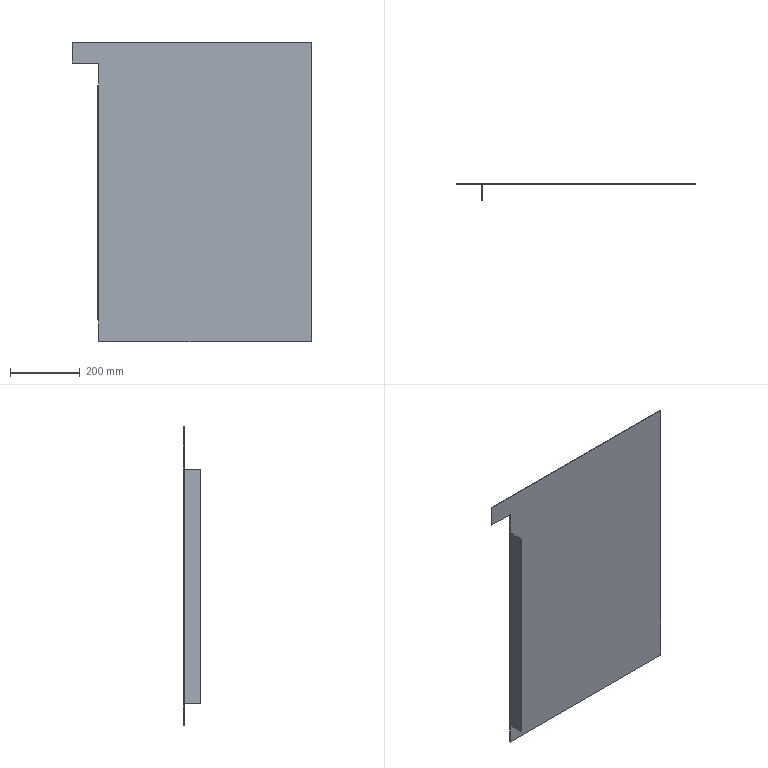Part | STEP file | 楼梯踏Plate 3 | 1 solid | 16 faces | box 686 x 50 x 860 mm | volume 1690832 mm3 | plane 14 | cylinder 2 | commonest cylinder face diameters 2 x1 8 x1
STEP:
#1=CARTESIAN_POINT('',(0.,0.,0.));
#2=DIRECTION('',(0.,0.,1.));
#3=DIRECTION('',(1.,0.,0.));
#4=AXIS2_PLACEMENT_3D('',#1,#2,#3);
#5=CARTESIAN_POINT('',(-611.,-3.,337.));
#6=VERTEX_POINT('',#5);
#7=CARTESIAN_POINT('',(-611.,-3.,-337.));
#8=VERTEX_POINT('',#7);
#9=CARTESIAN_POINT('',(-611.,-3.,337.));
#10=DIRECTION('',(0.,0.,-1.));
#11=VECTOR('',#10,1.);
#12=LINE('',#9,#11);
#13=CARTESIAN_POINT('',(-611.,-3.,337.));
#14=DIRECTION('',(0.,1.,0.));
#15=DIRECTION('',(0.,0.,1.));
#16=AXIS2_PLACEMENT_3D('',#13,#14,#15);
#17=PLANE('',#16);
#18=CARTESIAN_POINT('',(0.,0.));
#19=DIRECTION('',(-1.,0.));
#20=VECTOR('',#19,1.);
#21=LINE('',#18,#20);
#22=(GEOMETRIC_REPRESENTATION_CONTEXT(2)PARAMETRIC_REPRESENTATION_CONTEXT()REPRESENTATION_CONTEXT('',''));
#23=DEFINITIONAL_REPRESENTATION('',(#21),#22);
#24=PCURVE('',#17,#23);
#25=CARTESIAN_POINT('',(-611.,-4.,337.));
#26=DIRECTION('',(0.,0.,-1.));
#27=DIRECTION('',(-1.,0.,0.));
#28=AXIS2_PLACEMENT_3D('',#25,#26,#27);
#29=CYLINDRICAL_SURFACE('',#28,1.);
#30=CARTESIAN_POINT('',(1.571,0.));
#31=DIRECTION('',(0.,1.));
#32=VECTOR('',#31,1.);
#33=LINE('',#30,#32);
#34=(GEOMETRIC_REPRESENTATION_CONTEXT(2)PARAMETRIC_REPRESENTATION_CONTEXT()REPRESENTATION_CONTEXT('',''));
#35=DEFINITIONAL_REPRESENTATION('',(#33),#34);
#36=PCURVE('',#29,#35);
#37=SURFACE_CURVE('',#12,(#24,#36),.PCURVE_S1.);
#38=EDGE_CURVE('',#6,#8,#37,.T.);
#39=ORIENTED_EDGE('',*,*,#38,.T.);
#40=CARTESIAN_POINT('',(-611.,-3.,-400.));
#41=VERTEX_POINT('',#40);
#42=CARTESIAN_POINT('',(-611.,-3.,-337.));
#43=DIRECTION('',(0.,0.,1.));
#44=VECTOR('',#43,1.);
#45=LINE('',#42,#44);
#46=CARTESIAN_POINT('',(-674.,0.));
#47=DIRECTION('',(1.,0.));
#48=VECTOR('',#47,1.);
#49=LINE('',#46,#48);
#50=(GEOMETRIC_REPRESENTATION_CONTEXT(2)PARAMETRIC_REPRESENTATION_CONTEXT()REPRESENTATION_CONTEXT('',''));
#51=DEFINITIONAL_REPRESENTATION('',(#49),#50);
#52=PCURVE('',#17,#51);
#53=CARTESIAN_POINT('',(-611.,-3.,-337.));
#54=DIRECTION('',(-1.,0.,0.));
#55=DIRECTION('',(0.,0.,1.));
#56=AXIS2_PLACEMENT_3D('',#53,#54,#55);
#57=PLANE('',#56);
#58=CARTESIAN_POINT('',(0.,0.));
#59=DIRECTION('',(1.,0.));
#60=VECTOR('',#59,1.);
#61=LINE('',#58,#60);
#62=(GEOMETRIC_REPRESENTATION_CONTEXT(2)PARAMETRIC_REPRESENTATION_CONTEXT()REPRESENTATION_CONTEXT('',''));
#63=DEFINITIONAL_REPRESENTATION('',(#61),#62);
#64=PCURVE('',#57,#63);
#65=SURFACE_CURVE('',#45,(#52,#64),.PCURVE_S1.);
#66=EDGE_CURVE('',#41,#8,#65,.T.);
#67=ORIENTED_EDGE('',*,*,#66,.F.);
#68=CARTESIAN_POINT('',(0.,-3.,-400.));
#69=VERTEX_POINT('',#68);
#70=CARTESIAN_POINT('',(-611.,-3.,-400.));
#71=DIRECTION('',(-1.,0.,0.));
#72=VECTOR('',#71,1.);
#73=LINE('',#70,#72);
#74=CARTESIAN_POINT('',(-737.,0.));
#75=DIRECTION('',(0.,-1.));
#76=VECTOR('',#75,1.);
#77=LINE('',#74,#76);
#78=(GEOMETRIC_REPRESENTATION_CONTEXT(2)PARAMETRIC_REPRESENTATION_CONTEXT()REPRESENTATION_CONTEXT('',''));
#79=DEFINITIONAL_REPRESENTATION('',(#77),#78);
#80=PCURVE('',#17,#79);
#81=CARTESIAN_POINT('',(-611.,-3.,-400.));
#82=DIRECTION('',(0.,0.,-1.));
#83=DIRECTION('',(-1.,0.,0.));
#84=AXIS2_PLACEMENT_3D('',#81,#82,#83);
#85=PLANE('',#84);
#86=CARTESIAN_POINT('',(0.,0.));
#87=DIRECTION('',(1.,0.));
#88=VECTOR('',#87,1.);
#89=LINE('',#86,#88);
#90=(GEOMETRIC_REPRESENTATION_CONTEXT(2)PARAMETRIC_REPRESENTATION_CONTEXT()REPRESENTATION_CONTEXT('',''));
#91=DEFINITIONAL_REPRESENTATION('',(#89),#90);
#92=PCURVE('',#85,#91);
#93=SURFACE_CURVE('',#73,(#80,#92),.PCURVE_S1.);
#94=EDGE_CURVE('',#69,#41,#93,.T.);
#95=ORIENTED_EDGE('',*,*,#94,.F.);
#96=CARTESIAN_POINT('',(0.,-3.,460.));
#97=VERTEX_POINT('',#96);
#98=CARTESIAN_POINT('',(0.,-3.,337.));
#99=DIRECTION('',(0.,0.,-1.));
#100=VECTOR('',#99,1.);
#101=LINE('',#98,#100);
#102=CARTESIAN_POINT('',(0.,611.));
#103=DIRECTION('',(-1.,0.));
#104=VECTOR('',#103,1.);
#105=LINE('',#102,#104);
#106=(GEOMETRIC_REPRESENTATION_CONTEXT(2)PARAMETRIC_REPRESENTATION_CONTEXT()REPRESENTATION_CONTEXT('',''));
#107=DEFINITIONAL_REPRESENTATION('',(#105),#106);
#108=PCURVE('',#17,#107);
#109=CARTESIAN_POINT('',(0.,0.,337.));
#110=DIRECTION('',(1.,0.,0.));
#111=DIRECTION('',(0.,0.,-1.));
#112=AXIS2_PLACEMENT_3D('',#109,#110,#111);
#113=PLANE('',#112);
#114=CARTESIAN_POINT('',(0.,-3.));
#115=DIRECTION('',(1.,0.));
#116=VECTOR('',#115,1.);
#117=LINE('',#114,#116);
#118=(GEOMETRIC_REPRESENTATION_CONTEXT(2)PARAMETRIC_REPRESENTATION_CONTEXT()REPRESENTATION_CONTEXT('',''));
#119=DEFINITIONAL_REPRESENTATION('',(#117),#118);
#120=PCURVE('',#113,#119);
#121=SURFACE_CURVE('',#101,(#108,#120),.PCURVE_S1.);
#122=EDGE_CURVE('',#97,#69,#121,.T.);
#123=ORIENTED_EDGE('',*,*,#122,.F.);
#124=CARTESIAN_POINT('',(-686.,-3.,460.));
#125=VERTEX_POINT('',#124);
#126=CARTESIAN_POINT('',(-611.,-3.,460.));
#127=DIRECTION('',(1.,0.,0.));
#128=VECTOR('',#127,1.);
#129=LINE('',#126,#128);
#130=CARTESIAN_POINT('',(123.,0.));
#131=DIRECTION('',(0.,1.));
#132=VECTOR('',#131,1.);
#133=LINE('',#130,#132);
#134=(GEOMETRIC_REPRESENTATION_CONTEXT(2)PARAMETRIC_REPRESENTATION_CONTEXT()REPRESENTATION_CONTEXT('',''));
#135=DEFINITIONAL_REPRESENTATION('',(#133),#134);
#136=PCURVE('',#17,#135);
#137=CARTESIAN_POINT('',(-611.,-3.,460.));
#138=DIRECTION('',(0.,0.,1.));
#139=DIRECTION('',(1.,0.,0.));
#140=AXIS2_PLACEMENT_3D('',#137,#138,#139);
#141=PLANE('',#140);
#142=CARTESIAN_POINT('',(0.,0.));
#143=DIRECTION('',(1.,0.));
#144=VECTOR('',#143,1.);
#145=LINE('',#142,#144);
#146=(GEOMETRIC_REPRESENTATION_CONTEXT(2)PARAMETRIC_REPRESENTATION_CONTEXT()REPRESENTATION_CONTEXT('',''));
#147=DEFINITIONAL_REPRESENTATION('',(#145),#146);
#148=PCURVE('',#141,#147);
#149=SURFACE_CURVE('',#129,(#136,#148),.PCURVE_S1.);
#150=EDGE_CURVE('',#125,#97,#149,.T.);
#151=ORIENTED_EDGE('',*,*,#150,.F.);
#152=CARTESIAN_POINT('',(-686.,-3.,400.));
#153=VERTEX_POINT('',#152);
#154=CARTESIAN_POINT('',(-686.,-3.,460.));
#155=DIRECTION('',(0.,0.,1.));
#156=VECTOR('',#155,1.);
#157=LINE('',#154,#156);
#158=CARTESIAN_POINT('',(123.,-75.));
#159=DIRECTION('',(1.,0.));
#160=VECTOR('',#159,1.);
#161=LINE('',#158,#160);
#162=(GEOMETRIC_REPRESENTATION_CONTEXT(2)PARAMETRIC_REPRESENTATION_CONTEXT()REPRESENTATION_CONTEXT('',''));
#163=DEFINITIONAL_REPRESENTATION('',(#161),#162);
#164=PCURVE('',#17,#163);
#165=CARTESIAN_POINT('',(-686.,-3.,460.));
#166=DIRECTION('',(-1.,0.,0.));
#167=DIRECTION('',(0.,0.,1.));
#168=AXIS2_PLACEMENT_3D('',#165,#166,#167);
#169=PLANE('',#168);
#170=CARTESIAN_POINT('',(0.,0.));
#171=DIRECTION('',(1.,0.));
#172=VECTOR('',#171,1.);
#173=LINE('',#170,#172);
#174=(GEOMETRIC_REPRESENTATION_CONTEXT(2)PARAMETRIC_REPRESENTATION_CONTEXT()REPRESENTATION_CONTEXT('',''));
#175=DEFINITIONAL_REPRESENTATION('',(#173),#174);
#176=PCURVE('',#169,#175);
#177=SURFACE_CURVE('',#157,(#164,#176),.PCURVE_S1.);
#178=EDGE_CURVE('',#153,#125,#177,.T.);
#179=ORIENTED_EDGE('',*,*,#178,.F.);
#180=CARTESIAN_POINT('',(-611.,-3.,400.));
#181=VERTEX_POINT('',#180);
#182=CARTESIAN_POINT('',(-611.,-3.,400.));
#183=DIRECTION('',(-1.,0.,0.));
#184=VECTOR('',#183,1.);
#185=LINE('',#182,#184);
#186=CARTESIAN_POINT('',(63.,0.));
#187=DIRECTION('',(0.,-1.));
#188=VECTOR('',#187,1.);
#189=LINE('',#186,#188);
#190=(GEOMETRIC_REPRESENTATION_CONTEXT(2)PARAMETRIC_REPRESENTATION_CONTEXT()REPRESENTATION_CONTEXT('',''));
#191=DEFINITIONAL_REPRESENTATION('',(#189),#190);
#192=PCURVE('',#17,#191);
#193=CARTESIAN_POINT('',(-611.,-3.,400.));
#194=DIRECTION('',(0.,0.,-1.));
#195=DIRECTION('',(-1.,0.,0.));
#196=AXIS2_PLACEMENT_3D('',#193,#194,#195);
#197=PLANE('',#196);
#198=CARTESIAN_POINT('',(0.,0.));
#199=DIRECTION('',(1.,0.));
#200=VECTOR('',#199,1.);
#201=LINE('',#198,#200);
#202=(GEOMETRIC_REPRESENTATION_CONTEXT(2)PARAMETRIC_REPRESENTATION_CONTEXT()REPRESENTATION_CONTEXT('',''));
#203=DEFINITIONAL_REPRESENTATION('',(#201),#202);
#204=PCURVE('',#197,#203);
#205=SURFACE_CURVE('',#185,(#192,#204),.PCURVE_S1.);
#206=EDGE_CURVE('',#181,#153,#205,.T.);
#207=ORIENTED_EDGE('',*,*,#206,.F.);
#208=CARTESIAN_POINT('',(-611.,-3.,337.));
#209=DIRECTION('',(0.,0.,1.));
#210=VECTOR('',#209,1.);
#211=LINE('',#208,#210);
#212=CARTESIAN_POINT('',(0.,0.));
#213=DIRECTION('',(1.,0.));
#214=VECTOR('',#213,1.);
#215=LINE('',#212,#214);
#216=(GEOMETRIC_REPRESENTATION_CONTEXT(2)PARAMETRIC_REPRESENTATION_CONTEXT()REPRESENTATION_CONTEXT('',''));
#217=DEFINITIONAL_REPRESENTATION('',(#215),#216);
#218=PCURVE('',#17,#217);
#219=CARTESIAN_POINT('',(-611.,-3.,337.));
#220=DIRECTION('',(-1.,0.,0.));
#221=DIRECTION('',(0.,0.,1.));
#222=AXIS2_PLACEMENT_3D('',#219,#220,#221);
#223=PLANE('',#222);
#224=CARTESIAN_POINT('',(0.,0.));
#225=DIRECTION('',(1.,0.));
#226=VECTOR('',#225,1.);
#227=LINE('',#224,#226);
#228=(GEOMETRIC_REPRESENTATION_CONTEXT(2)PARAMETRIC_REPRESENTATION_CONTEXT()REPRESENTATION_CONTEXT('',''));
#229=DEFINITIONAL_REPRESENTATION('',(#227),#228);
#230=PCURVE('',#223,#229);
#231=SURFACE_CURVE('',#211,(#218,#230),.PCURVE_S1.);
#232=EDGE_CURVE('',#6,#181,#231,.T.);
#233=ORIENTED_EDGE('',*,*,#232,.F.);
#234=EDGE_LOOP('',(#39,#67,#95,#123,#151,#179,#207,#233));
#235=FACE_BOUND('',#234,.T.);
#236=ADVANCED_FACE('',(#235),#17,.F.);
#237=ORIENTED_EDGE('',*,*,#122,.T.);
#238=CARTESIAN_POINT('',(0.,0.,-400.));
#239=VERTEX_POINT('',#238);
#240=CARTESIAN_POINT('',(0.,-3.,-400.));
#241=DIRECTION('',(0.,1.,0.));
#242=VECTOR('',#241,1.);
#243=LINE('',#240,#242);
#244=CARTESIAN_POINT('',(737.,-3.));
#245=DIRECTION('',(0.,1.));
#246=VECTOR('',#245,1.);
#247=LINE('',#244,#246);
#248=(GEOMETRIC_REPRESENTATION_CONTEXT(2)PARAMETRIC_REPRESENTATION_CONTEXT()REPRESENTATION_CONTEXT('',''));
#249=DEFINITIONAL_REPRESENTATION('',(#247),#248);
#250=PCURVE('',#113,#249);
#251=CARTESIAN_POINT('',(-611.,0.));
#252=DIRECTION('',(0.,1.));
#253=VECTOR('',#252,1.);
#254=LINE('',#251,#253);
#255=(GEOMETRIC_REPRESENTATION_CONTEXT(2)PARAMETRIC_REPRESENTATION_CONTEXT()REPRESENTATION_CONTEXT('',''));
#256=DEFINITIONAL_REPRESENTATION('',(#254),#255);
#257=PCURVE('',#85,#256);
#258=SURFACE_CURVE('',#243,(#250,#257),.PCURVE_S1.);
#259=EDGE_CURVE('',#69,#239,#258,.T.);
#260=ORIENTED_EDGE('',*,*,#259,.T.);
#261=CARTESIAN_POINT('',(0.,0.,460.));
#262=VERTEX_POINT('',#261);
#263=CARTESIAN_POINT('',(0.,0.,337.));
#264=DIRECTION('',(0.,0.,-1.));
#265=VECTOR('',#264,1.);
#266=LINE('',#263,#265);
#267=CARTESIAN_POINT('',(0.,0.));
#268=DIRECTION('',(1.,0.));
#269=VECTOR('',#268,1.);
#270=LINE('',#267,#269);
#271=(GEOMETRIC_REPRESENTATION_CONTEXT(2)PARAMETRIC_REPRESENTATION_CONTEXT()REPRESENTATION_CONTEXT('',''));
#272=DEFINITIONAL_REPRESENTATION('',(#270),#271);
#273=PCURVE('',#113,#272);
#274=CARTESIAN_POINT('',(-611.,0.,337.));
#275=DIRECTION('',(0.,1.,0.));
#276=DIRECTION('',(0.,0.,1.));
#277=AXIS2_PLACEMENT_3D('',#274,#275,#276);
#278=PLANE('',#277);
#279=CARTESIAN_POINT('',(0.,611.));
#280=DIRECTION('',(-1.,0.));
#281=VECTOR('',#280,1.);
#282=LINE('',#279,#281);
#283=(GEOMETRIC_REPRESENTATION_CONTEXT(2)PARAMETRIC_REPRESENTATION_CONTEXT()REPRESENTATION_CONTEXT('',''));
#284=DEFINITIONAL_REPRESENTATION('',(#282),#283);
#285=PCURVE('',#278,#284);
#286=SURFACE_CURVE('',#266,(#273,#285),.PCURVE_S1.);
#287=EDGE_CURVE('',#262,#239,#286,.T.);
#288=ORIENTED_EDGE('',*,*,#287,.F.);
#289=CARTESIAN_POINT('',(0.,-3.,460.));
#290=DIRECTION('',(0.,1.,0.));
#291=VECTOR('',#290,1.);
#292=LINE('',#289,#291);
#293=CARTESIAN_POINT('',(-123.,-3.));
#294=DIRECTION('',(0.,1.));
#295=VECTOR('',#294,1.);
#296=LINE('',#293,#295);
#297=(GEOMETRIC_REPRESENTATION_CONTEXT(2)PARAMETRIC_REPRESENTATION_CONTEXT()REPRESENTATION_CONTEXT('',''));
#298=DEFINITIONAL_REPRESENTATION('',(#296),#297);
#299=PCURVE('',#113,#298);
#300=CARTESIAN_POINT('',(611.,0.));
#301=DIRECTION('',(0.,1.));
#302=VECTOR('',#301,1.);
#303=LINE('',#300,#302);
#304=(GEOMETRIC_REPRESENTATION_CONTEXT(2)PARAMETRIC_REPRESENTATION_CONTEXT()REPRESENTATION_CONTEXT('',''));
#305=DEFINITIONAL_REPRESENTATION('',(#303),#304);
#306=PCURVE('',#141,#305);
#307=SURFACE_CURVE('',#292,(#299,#306),.PCURVE_S1.);
#308=EDGE_CURVE('',#97,#262,#307,.T.);
#309=ORIENTED_EDGE('',*,*,#308,.F.);
#310=EDGE_LOOP('',(#237,#260,#288,#309));
#311=FACE_BOUND('',#310,.T.);
#312=ADVANCED_FACE('',(#311),#113,.T.);
#313=ORIENTED_EDGE('',*,*,#287,.T.);
#314=CARTESIAN_POINT('',(-611.,0.,-400.));
#315=VERTEX_POINT('',#314);
#316=CARTESIAN_POINT('',(-611.,0.,-400.));
#317=DIRECTION('',(-1.,0.,0.));
#318=VECTOR('',#317,1.);
#319=LINE('',#316,#318);
#320=CARTESIAN_POINT('',(-737.,0.));
#321=DIRECTION('',(0.,-1.));
#322=VECTOR('',#321,1.);
#323=LINE('',#320,#322);
#324=(GEOMETRIC_REPRESENTATION_CONTEXT(2)PARAMETRIC_REPRESENTATION_CONTEXT()REPRESENTATION_CONTEXT('',''));
#325=DEFINITIONAL_REPRESENTATION('',(#323),#324);
#326=PCURVE('',#278,#325);
#327=CARTESIAN_POINT('',(0.,3.));
#328=DIRECTION('',(1.,0.));
#329=VECTOR('',#328,1.);
#330=LINE('',#327,#329);
#331=(GEOMETRIC_REPRESENTATION_CONTEXT(2)PARAMETRIC_REPRESENTATION_CONTEXT()REPRESENTATION_CONTEXT('',''));
#332=DEFINITIONAL_REPRESENTATION('',(#330),#331);
#333=PCURVE('',#85,#332);
#334=SURFACE_CURVE('',#319,(#326,#333),.PCURVE_S1.);
#335=EDGE_CURVE('',#239,#315,#334,.T.);
#336=ORIENTED_EDGE('',*,*,#335,.T.);
#337=CARTESIAN_POINT('',(-611.,0.,-337.));
#338=VERTEX_POINT('',#337);
#339=CARTESIAN_POINT('',(-611.,0.,-337.));
#340=DIRECTION('',(0.,0.,1.));
#341=VECTOR('',#340,1.);
#342=LINE('',#339,#341);
#343=CARTESIAN_POINT('',(-674.,0.));
#344=DIRECTION('',(1.,0.));
#345=VECTOR('',#344,1.);
#346=LINE('',#343,#345);
#347=(GEOMETRIC_REPRESENTATION_CONTEXT(2)PARAMETRIC_REPRESENTATION_CONTEXT()REPRESENTATION_CONTEXT('',''));
#348=DEFINITIONAL_REPRESENTATION('',(#346),#347);
#349=PCURVE('',#278,#348);
#350=CARTESIAN_POINT('',(0.,3.));
#351=DIRECTION('',(1.,0.));
#352=VECTOR('',#351,1.);
#353=LINE('',#350,#352);
#354=(GEOMETRIC_REPRESENTATION_CONTEXT(2)PARAMETRIC_REPRESENTATION_CONTEXT()REPRESENTATION_CONTEXT('',''));
#355=DEFINITIONAL_REPRESENTATION('',(#353),#354);
#356=PCURVE('',#57,#355);
#357=SURFACE_CURVE('',#342,(#349,#356),.PCURVE_S1.);
#358=EDGE_CURVE('',#315,#338,#357,.T.);
#359=ORIENTED_EDGE('',*,*,#358,.T.);
#360=CARTESIAN_POINT('',(-611.,0.,337.));
#361=VERTEX_POINT('',#360);
#362=CARTESIAN_POINT('',(-611.,0.,337.));
#363=DIRECTION('',(0.,0.,-1.));
#364=VECTOR('',#363,1.);
#365=LINE('',#362,#364);
#366=CARTESIAN_POINT('',(0.,0.));
#367=DIRECTION('',(-1.,0.));
#368=VECTOR('',#367,1.);
#369=LINE('',#366,#368);
#370=(GEOMETRIC_REPRESENTATION_CONTEXT(2)PARAMETRIC_REPRESENTATION_CONTEXT()REPRESENTATION_CONTEXT('',''));
#371=DEFINITIONAL_REPRESENTATION('',(#369),#370);
#372=PCURVE('',#278,#371);
#373=CARTESIAN_POINT('',(-611.,-4.,337.));
#374=DIRECTION('',(0.,0.,-1.));
#375=DIRECTION('',(-1.,0.,0.));
#376=AXIS2_PLACEMENT_3D('',#373,#374,#375);
#377=CYLINDRICAL_SURFACE('',#376,4.);
#378=CARTESIAN_POINT('',(1.571,0.));
#379=DIRECTION('',(0.,1.));
#380=VECTOR('',#379,1.);
#381=LINE('',#378,#380);
#382=(GEOMETRIC_REPRESENTATION_CONTEXT(2)PARAMETRIC_REPRESENTATION_CONTEXT()REPRESENTATION_CONTEXT('',''));
#383=DEFINITIONAL_REPRESENTATION('',(#381),#382);
#384=PCURVE('',#377,#383);
#385=SURFACE_CURVE('',#365,(#372,#384),.PCURVE_S1.);
#386=EDGE_CURVE('',#361,#338,#385,.T.);
#387=ORIENTED_EDGE('',*,*,#386,.F.);
#388=CARTESIAN_POINT('',(-611.,0.,400.));
#389=VERTEX_POINT('',#388);
#390=CARTESIAN_POINT('',(-611.,0.,337.));
#391=DIRECTION('',(0.,0.,1.));
#392=VECTOR('',#391,1.);
#393=LINE('',#390,#392);
#394=CARTESIAN_POINT('',(0.,0.));
#395=DIRECTION('',(1.,0.));
#396=VECTOR('',#395,1.);
#397=LINE('',#394,#396);
#398=(GEOMETRIC_REPRESENTATION_CONTEXT(2)PARAMETRIC_REPRESENTATION_CONTEXT()REPRESENTATION_CONTEXT('',''));
#399=DEFINITIONAL_REPRESENTATION('',(#397),#398);
#400=PCURVE('',#278,#399);
#401=CARTESIAN_POINT('',(0.,3.));
#402=DIRECTION('',(1.,0.));
#403=VECTOR('',#402,1.);
#404=LINE('',#401,#403);
#405=(GEOMETRIC_REPRESENTATION_CONTEXT(2)PARAMETRIC_REPRESENTATION_CONTEXT()REPRESENTATION_CONTEXT('',''));
#406=DEFINITIONAL_REPRESENTATION('',(#404),#405);
#407=PCURVE('',#223,#406);
#408=SURFACE_CURVE('',#393,(#400,#407),.PCURVE_S1.);
#409=EDGE_CURVE('',#361,#389,#408,.T.);
#410=ORIENTED_EDGE('',*,*,#409,.T.);
#411=CARTESIAN_POINT('',(-686.,0.,400.));
#412=VERTEX_POINT('',#411);
#413=CARTESIAN_POINT('',(-611.,0.,400.));
#414=DIRECTION('',(-1.,0.,0.));
#415=VECTOR('',#414,1.);
#416=LINE('',#413,#415);
#417=CARTESIAN_POINT('',(63.,0.));
#418=DIRECTION('',(0.,-1.));
#419=VECTOR('',#418,1.);
#420=LINE('',#417,#419);
#421=(GEOMETRIC_REPRESENTATION_CONTEXT(2)PARAMETRIC_REPRESENTATION_CONTEXT()REPRESENTATION_CONTEXT('',''));
#422=DEFINITIONAL_REPRESENTATION('',(#420),#421);
#423=PCURVE('',#278,#422);
#424=CARTESIAN_POINT('',(0.,3.));
#425=DIRECTION('',(1.,0.));
#426=VECTOR('',#425,1.);
#427=LINE('',#424,#426);
#428=(GEOMETRIC_REPRESENTATION_CONTEXT(2)PARAMETRIC_REPRESENTATION_CONTEXT()REPRESENTATION_CONTEXT('',''));
#429=DEFINITIONAL_REPRESENTATION('',(#427),#428);
#430=PCURVE('',#197,#429);
#431=SURFACE_CURVE('',#416,(#423,#430),.PCURVE_S1.);
#432=EDGE_CURVE('',#389,#412,#431,.T.);
#433=ORIENTED_EDGE('',*,*,#432,.T.);
#434=CARTESIAN_POINT('',(-686.,0.,460.));
#435=VERTEX_POINT('',#434);
#436=CARTESIAN_POINT('',(-686.,0.,460.));
#437=DIRECTION('',(0.,0.,1.));
#438=VECTOR('',#437,1.);
#439=LINE('',#436,#438);
#440=CARTESIAN_POINT('',(123.,-75.));
#441=DIRECTION('',(1.,0.));
#442=VECTOR('',#441,1.);
#443=LINE('',#440,#442);
#444=(GEOMETRIC_REPRESENTATION_CONTEXT(2)PARAMETRIC_REPRESENTATION_CONTEXT()REPRESENTATION_CONTEXT('',''));
#445=DEFINITIONAL_REPRESENTATION('',(#443),#444);
#446=PCURVE('',#278,#445);
#447=CARTESIAN_POINT('',(0.,3.));
#448=DIRECTION('',(1.,0.));
#449=VECTOR('',#448,1.);
#450=LINE('',#447,#449);
#451=(GEOMETRIC_REPRESENTATION_CONTEXT(2)PARAMETRIC_REPRESENTATION_CONTEXT()REPRESENTATION_CONTEXT('',''));
#452=DEFINITIONAL_REPRESENTATION('',(#450),#451);
#453=PCURVE('',#169,#452);
#454=SURFACE_CURVE('',#439,(#446,#453),.PCURVE_S1.);
#455=EDGE_CURVE('',#412,#435,#454,.T.);
#456=ORIENTED_EDGE('',*,*,#455,.T.);
#457=CARTESIAN_POINT('',(-611.,0.,460.));
#458=DIRECTION('',(1.,0.,0.));
#459=VECTOR('',#458,1.);
#460=LINE('',#457,#459);
#461=CARTESIAN_POINT('',(123.,0.));
#462=DIRECTION('',(0.,1.));
#463=VECTOR('',#462,1.);
#464=LINE('',#461,#463);
#465=(GEOMETRIC_REPRESENTATION_CONTEXT(2)PARAMETRIC_REPRESENTATION_CONTEXT()REPRESENTATION_CONTEXT('',''));
#466=DEFINITIONAL_REPRESENTATION('',(#464),#465);
#467=PCURVE('',#278,#466);
#468=CARTESIAN_POINT('',(0.,3.));
#469=DIRECTION('',(1.,0.));
#470=VECTOR('',#469,1.);
#471=LINE('',#468,#470);
#472=(GEOMETRIC_REPRESENTATION_CONTEXT(2)PARAMETRIC_REPRESENTATION_CONTEXT()REPRESENTATION_CONTEXT('',''));
#473=DEFINITIONAL_REPRESENTATION('',(#471),#472);
#474=PCURVE('',#141,#473);
#475=SURFACE_CURVE('',#460,(#467,#474),.PCURVE_S1.);
#476=EDGE_CURVE('',#435,#262,#475,.T.);
#477=ORIENTED_EDGE('',*,*,#476,.T.);
#478=EDGE_LOOP('',(#313,#336,#359,#387,#410,#433,#456,#477));
#479=FACE_BOUND('',#478,.T.);
#480=ADVANCED_FACE('',(#479),#278,.T.);
#481=CARTESIAN_POINT('',(-615.,-4.,-337.));
#482=VERTEX_POINT('',#481);
#483=CARTESIAN_POINT('',(-611.,-4.,-337.));
#484=DIRECTION('',(0.,0.,-1.));
#485=DIRECTION('',(1.,0.,0.));
#486=AXIS2_PLACEMENT_3D('',#483,#484,#485);
#487=CIRCLE('',#486,4.);
#488=CARTESIAN_POINT('',(-3.142,674.));
#489=DIRECTION('',(1.,0.));
#490=VECTOR('',#489,1.);
#491=LINE('',#488,#490);
#492=(GEOMETRIC_REPRESENTATION_CONTEXT(2)PARAMETRIC_REPRESENTATION_CONTEXT()REPRESENTATION_CONTEXT('',''));
#493=DEFINITIONAL_REPRESENTATION('',(#491),#492);
#494=PCURVE('',#377,#493);
#495=CARTESIAN_POINT('',(-611.,-4.,-337.));
#496=DIRECTION('',(0.,0.,-1.));
#497=DIRECTION('',(-1.,0.,0.));
#498=AXIS2_PLACEMENT_3D('',#495,#496,#497);
#499=PLANE('',#498);
#500=CARTESIAN_POINT('',(0.,0.));
#501=DIRECTION('',(-1.,0.));
#502=AXIS2_PLACEMENT_2D('',#500,#501);
#503=CIRCLE('',#502,4.);
#504=(GEOMETRIC_REPRESENTATION_CONTEXT(2)PARAMETRIC_REPRESENTATION_CONTEXT()REPRESENTATION_CONTEXT('',''));
#505=DEFINITIONAL_REPRESENTATION('',(#503),#504);
#506=PCURVE('',#499,#505);
#507=SURFACE_CURVE('',#487,(#494,#506),.PCURVE_S1.);
#508=EDGE_CURVE('',#482,#338,#507,.T.);
#509=ORIENTED_EDGE('',*,*,#508,.F.);
#510=CARTESIAN_POINT('',(-615.,-4.,337.));
#511=VERTEX_POINT('',#510);
#512=CARTESIAN_POINT('',(-615.,-4.,337.));
#513=DIRECTION('',(0.,0.,-1.));
#514=VECTOR('',#513,1.);
#515=LINE('',#512,#514);
#516=CARTESIAN_POINT('',(0.,0.));
#517=DIRECTION('',(0.,1.));
#518=VECTOR('',#517,1.);
#519=LINE('',#516,#518);
#520=(GEOMETRIC_REPRESENTATION_CONTEXT(2)PARAMETRIC_REPRESENTATION_CONTEXT()REPRESENTATION_CONTEXT('',''));
#521=DEFINITIONAL_REPRESENTATION('',(#519),#520);
#522=PCURVE('',#377,#521);
#523=CARTESIAN_POINT('',(-615.,-4.,337.));
#524=DIRECTION('',(-1.,0.,0.));
#525=DIRECTION('',(0.,0.,1.));
#526=AXIS2_PLACEMENT_3D('',#523,#524,#525);
#527=PLANE('',#526);
#528=CARTESIAN_POINT('',(0.,0.));
#529=DIRECTION('',(-1.,0.));
#530=VECTOR('',#529,1.);
#531=LINE('',#528,#530);
#532=(GEOMETRIC_REPRESENTATION_CONTEXT(2)PARAMETRIC_REPRESENTATION_CONTEXT()REPRESENTATION_CONTEXT('',''));
#533=DEFINITIONAL_REPRESENTATION('',(#531),#532);
#534=PCURVE('',#527,#533);
#535=SURFACE_CURVE('',#515,(#522,#534),.PCURVE_S1.);
#536=EDGE_CURVE('',#511,#482,#535,.T.);
#537=ORIENTED_EDGE('',*,*,#536,.F.);
#538=CARTESIAN_POINT('',(-611.,-4.,337.));
#539=DIRECTION('',(0.,0.,-1.));
#540=DIRECTION('',(1.,0.,0.));
#541=AXIS2_PLACEMENT_3D('',#538,#539,#540);
#542=CIRCLE('',#541,4.);
#543=CARTESIAN_POINT('',(-3.142,0.));
#544=DIRECTION('',(1.,0.));
#545=VECTOR('',#544,1.);
#546=LINE('',#543,#545);
#547=(GEOMETRIC_REPRESENTATION_CONTEXT(2)PARAMETRIC_REPRESENTATION_CONTEXT()REPRESENTATION_CONTEXT('',''));
#548=DEFINITIONAL_REPRESENTATION('',(#546),#547);
#549=PCURVE('',#377,#548);
#550=CARTESIAN_POINT('',(-611.,-4.,337.));
#551=DIRECTION('',(0.,0.,-1.));
#552=DIRECTION('',(-1.,0.,0.));
#553=AXIS2_PLACEMENT_3D('',#550,#551,#552);
#554=PLANE('',#553);
#555=CARTESIAN_POINT('',(0.,0.));
#556=DIRECTION('',(-1.,0.));
#557=AXIS2_PLACEMENT_2D('',#555,#556);
#558=CIRCLE('',#557,4.);
#559=(GEOMETRIC_REPRESENTATION_CONTEXT(2)PARAMETRIC_REPRESENTATION_CONTEXT()REPRESENTATION_CONTEXT('',''));
#560=DEFINITIONAL_REPRESENTATION('',(#558),#559);
#561=PCURVE('',#554,#560);
#562=SURFACE_CURVE('',#542,(#549,#561),.PCURVE_S1.);
#563=EDGE_CURVE('',#511,#361,#562,.T.);
#564=ORIENTED_EDGE('',*,*,#563,.T.);
#565=ORIENTED_EDGE('',*,*,#386,.T.);
#566=EDGE_LOOP('',(#509,#537,#564,#565));
#567=FACE_BOUND('',#566,.T.);
#568=ADVANCED_FACE('',(#567),#377,.T.);
#569=CARTESIAN_POINT('',(-615.,-50.,-337.));
#570=VERTEX_POINT('',#569);
#571=CARTESIAN_POINT('',(-615.,-4.,-337.));
#572=DIRECTION('',(0.,1.,0.));
#573=VECTOR('',#572,1.);
#574=LINE('',#571,#573);
#575=CARTESIAN_POINT('',(-674.,0.));
#576=DIRECTION('',(0.,1.));
#577=VECTOR('',#576,1.);
#578=LINE('',#575,#577);
#579=(GEOMETRIC_REPRESENTATION_CONTEXT(2)PARAMETRIC_REPRESENTATION_CONTEXT()REPRESENTATION_CONTEXT('',''));
#580=DEFINITIONAL_REPRESENTATION('',(#578),#579);
#581=PCURVE('',#527,#580);
#582=CARTESIAN_POINT('',(4.,0.));
#583=DIRECTION('',(0.,1.));
#584=VECTOR('',#583,1.);
#585=LINE('',#582,#584);
#586=(GEOMETRIC_REPRESENTATION_CONTEXT(2)PARAMETRIC_REPRESENTATION_CONTEXT()REPRESENTATION_CONTEXT('',''));
#587=DEFINITIONAL_REPRESENTATION('',(#585),#586);
#588=PCURVE('',#499,#587);
#589=SURFACE_CURVE('',#574,(#581,#588),.PCURVE_S1.);
#590=EDGE_CURVE('',#570,#482,#589,.T.);
#591=ORIENTED_EDGE('',*,*,#590,.F.);
#592=CARTESIAN_POINT('',(-615.,-50.,337.));
#593=VERTEX_POINT('',#592);
#594=CARTESIAN_POINT('',(-615.,-50.,337.));
#595=DIRECTION('',(0.,0.,-1.));
#596=VECTOR('',#595,1.);
#597=LINE('',#594,#596);
#598=CARTESIAN_POINT('',(0.,-46.));
#599=DIRECTION('',(-1.,0.));
#600=VECTOR('',#599,1.);
#601=LINE('',#598,#600);
#602=(GEOMETRIC_REPRESENTATION_CONTEXT(2)PARAMETRIC_REPRESENTATION_CONTEXT()REPRESENTATION_CONTEXT('',''));
#603=DEFINITIONAL_REPRESENTATION('',(#601),#602);
#604=PCURVE('',#527,#603);
#605=CARTESIAN_POINT('',(-612.,-50.,337.));
#606=DIRECTION('',(0.,-1.,0.));
#607=DIRECTION('',(0.,0.,-1.));
#608=AXIS2_PLACEMENT_3D('',#605,#606,#607);
#609=PLANE('',#608);
#610=CARTESIAN_POINT('',(0.,-3.));
#611=DIRECTION('',(1.,0.));
#612=VECTOR('',#611,1.);
#613=LINE('',#610,#612);
#614=(GEOMETRIC_REPRESENTATION_CONTEXT(2)PARAMETRIC_REPRESENTATION_CONTEXT()REPRESENTATION_CONTEXT('',''));
#615=DEFINITIONAL_REPRESENTATION('',(#613),#614);
#616=PCURVE('',#609,#615);
#617=SURFACE_CURVE('',#597,(#604,#616),.PCURVE_S1.);
#618=EDGE_CURVE('',#593,#570,#617,.T.);
#619=ORIENTED_EDGE('',*,*,#618,.F.);
#620=CARTESIAN_POINT('',(-615.,-4.,337.));
#621=DIRECTION('',(0.,1.,0.));
#622=VECTOR('',#621,1.);
#623=LINE('',#620,#622);
#624=CARTESIAN_POINT('',(0.,0.));
#625=DIRECTION('',(0.,1.));
#626=VECTOR('',#625,1.);
#627=LINE('',#624,#626);
#628=(GEOMETRIC_REPRESENTATION_CONTEXT(2)PARAMETRIC_REPRESENTATION_CONTEXT()REPRESENTATION_CONTEXT('',''));
#629=DEFINITIONAL_REPRESENTATION('',(#627),#628);
#630=PCURVE('',#527,#629);
#631=CARTESIAN_POINT('',(4.,0.));
#632=DIRECTION('',(0.,1.));
#633=VECTOR('',#632,1.);
#634=LINE('',#631,#633);
#635=(GEOMETRIC_REPRESENTATION_CONTEXT(2)PARAMETRIC_REPRESENTATION_CONTEXT()REPRESENTATION_CONTEXT('',''));
#636=DEFINITIONAL_REPRESENTATION('',(#634),#635);
#637=PCURVE('',#554,#636);
#638=SURFACE_CURVE('',#623,(#630,#637),.PCURVE_S1.);
#639=EDGE_CURVE('',#593,#511,#638,.T.);
#640=ORIENTED_EDGE('',*,*,#639,.T.);
#641=ORIENTED_EDGE('',*,*,#536,.T.);
#642=EDGE_LOOP('',(#591,#619,#640,#641));
#643=FACE_BOUND('',#642,.T.);
#644=ADVANCED_FACE('',(#643),#527,.T.);
#645=CARTESIAN_POINT('',(-612.,-50.,-337.));
#646=VERTEX_POINT('',#645);
#647=CARTESIAN_POINT('',(-612.,-50.,-337.));
#648=DIRECTION('',(-1.,0.,0.));
#649=VECTOR('',#648,1.);
#650=LINE('',#647,#649);
#651=CARTESIAN_POINT('',(674.,0.));
#652=DIRECTION('',(0.,-1.));
#653=VECTOR('',#652,1.);
#654=LINE('',#651,#653);
#655=(GEOMETRIC_REPRESENTATION_CONTEXT(2)PARAMETRIC_REPRESENTATION_CONTEXT()REPRESENTATION_CONTEXT('',''));
#656=DEFINITIONAL_REPRESENTATION('',(#654),#655);
#657=PCURVE('',#609,#656);
#658=CARTESIAN_POINT('',(1.,-46.));
#659=DIRECTION('',(1.,0.));
#660=VECTOR('',#659,1.);
#661=LINE('',#658,#660);
#662=(GEOMETRIC_REPRESENTATION_CONTEXT(2)PARAMETRIC_REPRESENTATION_CONTEXT()REPRESENTATION_CONTEXT('',''));
#663=DEFINITIONAL_REPRESENTATION('',(#661),#662);
#664=PCURVE('',#499,#663);
#665=SURFACE_CURVE('',#650,(#657,#664),.PCURVE_S1.);
#666=EDGE_CURVE('',#646,#570,#665,.T.);
#667=ORIENTED_EDGE('',*,*,#666,.F.);
#668=CARTESIAN_POINT('',(-612.,-50.,337.));
#669=VERTEX_POINT('',#668);
#670=CARTESIAN_POINT('',(-612.,-50.,337.));
#671=DIRECTION('',(0.,0.,-1.));
#672=VECTOR('',#671,1.);
#673=LINE('',#670,#672);
#674=CARTESIAN_POINT('',(0.,0.));
#675=DIRECTION('',(1.,0.));
#676=VECTOR('',#675,1.);
#677=LINE('',#674,#676);
#678=(GEOMETRIC_REPRESENTATION_CONTEXT(2)PARAMETRIC_REPRESENTATION_CONTEXT()REPRESENTATION_CONTEXT('',''));
#679=DEFINITIONAL_REPRESENTATION('',(#677),#678);
#680=PCURVE('',#609,#679);
#681=CARTESIAN_POINT('',(-612.,-4.,337.));
#682=DIRECTION('',(-1.,0.,0.));
#683=DIRECTION('',(0.,0.,1.));
#684=AXIS2_PLACEMENT_3D('',#681,#682,#683);
#685=PLANE('',#684);
#686=CARTESIAN_POINT('',(0.,-46.));
#687=DIRECTION('',(-1.,0.));
#688=VECTOR('',#687,1.);
#689=LINE('',#686,#688);
#690=(GEOMETRIC_REPRESENTATION_CONTEXT(2)PARAMETRIC_REPRESENTATION_CONTEXT()REPRESENTATION_CONTEXT('',''));
#691=DEFINITIONAL_REPRESENTATION('',(#689),#690);
#692=PCURVE('',#685,#691);
#693=SURFACE_CURVE('',#673,(#680,#692),.PCURVE_S1.);
#694=EDGE_CURVE('',#669,#646,#693,.T.);
#695=ORIENTED_EDGE('',*,*,#694,.F.);
#696=CARTESIAN_POINT('',(-612.,-50.,337.));
#697=DIRECTION('',(-1.,0.,0.));
#698=VECTOR('',#697,1.);
#699=LINE('',#696,#698);
#700=CARTESIAN_POINT('',(0.,0.));
#701=DIRECTION('',(0.,-1.));
#702=VECTOR('',#701,1.);
#703=LINE('',#700,#702);
#704=(GEOMETRIC_REPRESENTATION_CONTEXT(2)PARAMETRIC_REPRESENTATION_CONTEXT()REPRESENTATION_CONTEXT('',''));
#705=DEFINITIONAL_REPRESENTATION('',(#703),#704);
#706=PCURVE('',#609,#705);
#707=CARTESIAN_POINT('',(1.,-46.));
#708=DIRECTION('',(1.,0.));
#709=VECTOR('',#708,1.);
#710=LINE('',#707,#709);
#711=(GEOMETRIC_REPRESENTATION_CONTEXT(2)PARAMETRIC_REPRESENTATION_CONTEXT()REPRESENTATION_CONTEXT('',''));
#712=DEFINITIONAL_REPRESENTATION('',(#710),#711);
#713=PCURVE('',#554,#712);
#714=SURFACE_CURVE('',#699,(#706,#713),.PCURVE_S1.);
#715=EDGE_CURVE('',#669,#593,#714,.T.);
#716=ORIENTED_EDGE('',*,*,#715,.T.);
#717=ORIENTED_EDGE('',*,*,#618,.T.);
#718=EDGE_LOOP('',(#667,#695,#716,#717));
#719=FACE_BOUND('',#718,.T.);
#720=ADVANCED_FACE('',(#719),#609,.T.);
#721=CARTESIAN_POINT('',(-612.,-4.,-337.));
#722=VERTEX_POINT('',#721);
#723=CARTESIAN_POINT('',(-612.,-4.,-337.));
#724=DIRECTION('',(0.,1.,0.));
#725=VECTOR('',#724,1.);
#726=LINE('',#723,#725);
#727=CARTESIAN_POINT('',(-674.,0.));
#728=DIRECTION('',(0.,1.));
#729=VECTOR('',#728,1.);
#730=LINE('',#727,#729);
#731=(GEOMETRIC_REPRESENTATION_CONTEXT(2)PARAMETRIC_REPRESENTATION_CONTEXT()REPRESENTATION_CONTEXT('',''));
#732=DEFINITIONAL_REPRESENTATION('',(#730),#731);
#733=PCURVE('',#685,#732);
#734=CARTESIAN_POINT('',(1.,0.));
#735=DIRECTION('',(0.,1.));
#736=VECTOR('',#735,1.);
#737=LINE('',#734,#736);
#738=(GEOMETRIC_REPRESENTATION_CONTEXT(2)PARAMETRIC_REPRESENTATION_CONTEXT()REPRESENTATION_CONTEXT('',''));
#739=DEFINITIONAL_REPRESENTATION('',(#737),#738);
#740=PCURVE('',#499,#739);
#741=SURFACE_CURVE('',#726,(#733,#740),.PCURVE_S1.);
#742=EDGE_CURVE('',#646,#722,#741,.T.);
#743=ORIENTED_EDGE('',*,*,#742,.T.);
#744=CARTESIAN_POINT('',(-612.,-4.,337.));
#745=VERTEX_POINT('',#744);
#746=CARTESIAN_POINT('',(-612.,-4.,337.));
#747=DIRECTION('',(0.,0.,-1.));
#748=VECTOR('',#747,1.);
#749=LINE('',#746,#748);
#750=CARTESIAN_POINT('',(0.,0.));
#751=DIRECTION('',(-1.,0.));
#752=VECTOR('',#751,1.);
#753=LINE('',#750,#752);
#754=(GEOMETRIC_REPRESENTATION_CONTEXT(2)PARAMETRIC_REPRESENTATION_CONTEXT()REPRESENTATION_CONTEXT('',''));
#755=DEFINITIONAL_REPRESENTATION('',(#753),#754);
#756=PCURVE('',#685,#755);
#757=CARTESIAN_POINT('',(0.,0.));
#758=DIRECTION('',(0.,1.));
#759=VECTOR('',#758,1.);
#760=LINE('',#757,#759);
#761=(GEOMETRIC_REPRESENTATION_CONTEXT(2)PARAMETRIC_REPRESENTATION_CONTEXT()REPRESENTATION_CONTEXT('',''));
#762=DEFINITIONAL_REPRESENTATION('',(#760),#761);
#763=PCURVE('',#29,#762);
#764=SURFACE_CURVE('',#749,(#756,#763),.PCURVE_S1.);
#765=EDGE_CURVE('',#745,#722,#764,.T.);
#766=ORIENTED_EDGE('',*,*,#765,.F.);
#767=CARTESIAN_POINT('',(-612.,-4.,337.));
#768=DIRECTION('',(0.,1.,0.));
#769=VECTOR('',#768,1.);
#770=LINE('',#767,#769);
#771=CARTESIAN_POINT('',(0.,0.));
#772=DIRECTION('',(0.,1.));
#773=VECTOR('',#772,1.);
#774=LINE('',#771,#773);
#775=(GEOMETRIC_REPRESENTATION_CONTEXT(2)PARAMETRIC_REPRESENTATION_CONTEXT()REPRESENTATION_CONTEXT('',''));
#776=DEFINITIONAL_REPRESENTATION('',(#774),#775);
#777=PCURVE('',#685,#776);
#778=CARTESIAN_POINT('',(1.,0.));
#779=DIRECTION('',(0.,1.));
#780=VECTOR('',#779,1.);
#781=LINE('',#778,#780);
#782=(GEOMETRIC_REPRESENTATION_CONTEXT(2)PARAMETRIC_REPRESENTATION_CONTEXT()REPRESENTATION_CONTEXT('',''));
#783=DEFINITIONAL_REPRESENTATION('',(#781),#782);
#784=PCURVE('',#554,#783);
#785=SURFACE_CURVE('',#770,(#777,#784),.PCURVE_S1.);
#786=EDGE_CURVE('',#669,#745,#785,.T.);
#787=ORIENTED_EDGE('',*,*,#786,.F.);
#788=ORIENTED_EDGE('',*,*,#694,.T.);
#789=EDGE_LOOP('',(#743,#766,#787,#788));
#790=FACE_BOUND('',#789,.T.);
#791=ADVANCED_FACE('',(#790),#685,.F.);
#792=ORIENTED_EDGE('',*,*,#765,.F.);
#793=CARTESIAN_POINT('',(-611.,-4.,337.));
#794=DIRECTION('',(0.,0.,-1.));
#795=DIRECTION('',(1.,0.,0.));
#796=AXIS2_PLACEMENT_3D('',#793,#794,#795);
#797=CIRCLE('',#796,1.);
#798=CARTESIAN_POINT('',(-3.142,0.));
#799=DIRECTION('',(1.,0.));
#800=VECTOR('',#799,1.);
#801=LINE('',#798,#800);
#802=(GEOMETRIC_REPRESENTATION_CONTEXT(2)PARAMETRIC_REPRESENTATION_CONTEXT()REPRESENTATION_CONTEXT('',''));
#803=DEFINITIONAL_REPRESENTATION('',(#801),#802);
#804=PCURVE('',#29,#803);
#805=CARTESIAN_POINT('',(0.,0.));
#806=DIRECTION('',(-1.,0.));
#807=AXIS2_PLACEMENT_2D('',#805,#806);
#808=CIRCLE('',#807,1.);
#809=(GEOMETRIC_REPRESENTATION_CONTEXT(2)PARAMETRIC_REPRESENTATION_CONTEXT()REPRESENTATION_CONTEXT('',''));
#810=DEFINITIONAL_REPRESENTATION('',(#808),#809);
#811=PCURVE('',#554,#810);
#812=SURFACE_CURVE('',#797,(#804,#811),.PCURVE_S1.);
#813=EDGE_CURVE('',#745,#6,#812,.T.);
#814=ORIENTED_EDGE('',*,*,#813,.T.);
#815=ORIENTED_EDGE('',*,*,#38,.T.);
#816=CARTESIAN_POINT('',(-611.,-4.,-337.));
#817=DIRECTION('',(0.,0.,-1.));
#818=DIRECTION('',(1.,0.,0.));
#819=AXIS2_PLACEMENT_3D('',#816,#817,#818);
#820=CIRCLE('',#819,1.);
#821=CARTESIAN_POINT('',(-3.142,674.));
#822=DIRECTION('',(1.,0.));
#823=VECTOR('',#822,1.);
#824=LINE('',#821,#823);
#825=(GEOMETRIC_REPRESENTATION_CONTEXT(2)PARAMETRIC_REPRESENTATION_CONTEXT()REPRESENTATION_CONTEXT('',''));
#826=DEFINITIONAL_REPRESENTATION('',(#824),#825);
#827=PCURVE('',#29,#826);
#828=CARTESIAN_POINT('',(0.,0.));
#829=DIRECTION('',(-1.,0.));
#830=AXIS2_PLACEMENT_2D('',#828,#829);
#831=CIRCLE('',#830,1.);
#832=(GEOMETRIC_REPRESENTATION_CONTEXT(2)PARAMETRIC_REPRESENTATION_CONTEXT()REPRESENTATION_CONTEXT('',''));
#833=DEFINITIONAL_REPRESENTATION('',(#831),#832);
#834=PCURVE('',#499,#833);
#835=SURFACE_CURVE('',#820,(#827,#834),.PCURVE_S1.);
#836=EDGE_CURVE('',#722,#8,#835,.T.);
#837=ORIENTED_EDGE('',*,*,#836,.F.);
#838=EDGE_LOOP('',(#792,#814,#815,#837));
#839=FACE_BOUND('',#838,.F.);
#840=ADVANCED_FACE('',(#839),#29,.F.);
#841=ORIENTED_EDGE('',*,*,#813,.T.);
#842=CARTESIAN_POINT('',(-611.,-3.,337.));
#843=DIRECTION('',(0.,1.,0.));
#844=VECTOR('',#843,1.);
#845=LINE('',#842,#844);
#846=CARTESIAN_POINT('',(0.,1.));
#847=DIRECTION('',(0.,1.));
#848=VECTOR('',#847,1.);
#849=LINE('',#846,#848);
#850=(GEOMETRIC_REPRESENTATION_CONTEXT(2)PARAMETRIC_REPRESENTATION_CONTEXT()REPRESENTATION_CONTEXT('',''));
#851=DEFINITIONAL_REPRESENTATION('',(#849),#850);
#852=PCURVE('',#554,#851);
#853=CARTESIAN_POINT('',(0.,0.));
#854=DIRECTION('',(0.,1.));
#855=VECTOR('',#854,1.);
#856=LINE('',#853,#855);
#857=(GEOMETRIC_REPRESENTATION_CONTEXT(2)PARAMETRIC_REPRESENTATION_CONTEXT()REPRESENTATION_CONTEXT('',''));
#858=DEFINITIONAL_REPRESENTATION('',(#856),#857);
#859=PCURVE('',#223,#858);
#860=SURFACE_CURVE('',#845,(#852,#859),.PCURVE_S1.);
#861=EDGE_CURVE('',#6,#361,#860,.T.);
#862=ORIENTED_EDGE('',*,*,#861,.T.);
#863=ORIENTED_EDGE('',*,*,#563,.F.);
#864=ORIENTED_EDGE('',*,*,#639,.F.);
#865=ORIENTED_EDGE('',*,*,#715,.F.);
#866=ORIENTED_EDGE('',*,*,#786,.T.);
#867=EDGE_LOOP('',(#841,#862,#863,#864,#865,#866));
#868=FACE_BOUND('',#867,.T.);
#869=ADVANCED_FACE('',(#868),#554,.F.);
#870=CARTESIAN_POINT('',(-611.,-3.,-337.));
#871=DIRECTION('',(0.,1.,0.));
#872=VECTOR('',#871,1.);
#873=LINE('',#870,#872);
#874=CARTESIAN_POINT('',(0.,1.));
#875=DIRECTION('',(0.,1.));
#876=VECTOR('',#875,1.);
#877=LINE('',#874,#876);
#878=(GEOMETRIC_REPRESENTATION_CONTEXT(2)PARAMETRIC_REPRESENTATION_CONTEXT()REPRESENTATION_CONTEXT('',''));
#879=DEFINITIONAL_REPRESENTATION('',(#877),#878);
#880=PCURVE('',#499,#879);
#881=CARTESIAN_POINT('',(0.,0.));
#882=DIRECTION('',(0.,1.));
#883=VECTOR('',#882,1.);
#884=LINE('',#881,#883);
#885=(GEOMETRIC_REPRESENTATION_CONTEXT(2)PARAMETRIC_REPRESENTATION_CONTEXT()REPRESENTATION_CONTEXT('',''));
#886=DEFINITIONAL_REPRESENTATION('',(#884),#885);
#887=PCURVE('',#57,#886);
#888=SURFACE_CURVE('',#873,(#880,#887),.PCURVE_S1.);
#889=EDGE_CURVE('',#8,#338,#888,.T.);
#890=ORIENTED_EDGE('',*,*,#889,.F.);
#891=ORIENTED_EDGE('',*,*,#836,.F.);
#892=ORIENTED_EDGE('',*,*,#742,.F.);
#893=ORIENTED_EDGE('',*,*,#666,.T.);
#894=ORIENTED_EDGE('',*,*,#590,.T.);
#895=ORIENTED_EDGE('',*,*,#508,.T.);
#896=EDGE_LOOP('',(#890,#891,#892,#893,#894,#895));
#897=FACE_BOUND('',#896,.T.);
#898=ADVANCED_FACE('',(#897),#499,.T.);
#899=ORIENTED_EDGE('',*,*,#358,.F.);
#900=CARTESIAN_POINT('',(-611.,-3.,-400.));
#901=DIRECTION('',(0.,1.,0.));
#902=VECTOR('',#901,1.);
#903=LINE('',#900,#902);
#904=CARTESIAN_POINT('',(-63.,0.));
#905=DIRECTION('',(0.,1.));
#906=VECTOR('',#905,1.);
#907=LINE('',#904,#906);
#908=(GEOMETRIC_REPRESENTATION_CONTEXT(2)PARAMETRIC_REPRESENTATION_CONTEXT()REPRESENTATION_CONTEXT('',''));
#909=DEFINITIONAL_REPRESENTATION('',(#907),#908);
#910=PCURVE('',#57,#909);
#911=CARTESIAN_POINT('',(0.,0.));
#912=DIRECTION('',(0.,1.));
#913=VECTOR('',#912,1.);
#914=LINE('',#911,#913);
#915=(GEOMETRIC_REPRESENTATION_CONTEXT(2)PARAMETRIC_REPRESENTATION_CONTEXT()REPRESENTATION_CONTEXT('',''));
#916=DEFINITIONAL_REPRESENTATION('',(#914),#915);
#917=PCURVE('',#85,#916);
#918=SURFACE_CURVE('',#903,(#910,#917),.PCURVE_S1.);
#919=EDGE_CURVE('',#41,#315,#918,.T.);
#920=ORIENTED_EDGE('',*,*,#919,.F.);
#921=ORIENTED_EDGE('',*,*,#66,.T.);
#922=ORIENTED_EDGE('',*,*,#889,.T.);
#923=EDGE_LOOP('',(#899,#920,#921,#922));
#924=FACE_BOUND('',#923,.T.);
#925=ADVANCED_FACE('',(#924),#57,.T.);
#926=ORIENTED_EDGE('',*,*,#335,.F.);
#927=ORIENTED_EDGE('',*,*,#259,.F.);
#928=ORIENTED_EDGE('',*,*,#94,.T.);
#929=ORIENTED_EDGE('',*,*,#919,.T.);
#930=EDGE_LOOP('',(#926,#927,#928,#929));
#931=FACE_BOUND('',#930,.T.);
#932=ADVANCED_FACE('',(#931),#85,.T.);
#933=CARTESIAN_POINT('',(-611.,-3.,400.));
#934=DIRECTION('',(0.,1.,0.));
#935=VECTOR('',#934,1.);
#936=LINE('',#933,#935);
#937=CARTESIAN_POINT('',(63.,0.));
#938=DIRECTION('',(0.,1.));
#939=VECTOR('',#938,1.);
#940=LINE('',#937,#939);
#941=(GEOMETRIC_REPRESENTATION_CONTEXT(2)PARAMETRIC_REPRESENTATION_CONTEXT()REPRESENTATION_CONTEXT('',''));
#942=DEFINITIONAL_REPRESENTATION('',(#940),#941);
#943=PCURVE('',#223,#942);
#944=CARTESIAN_POINT('',(0.,0.));
#945=DIRECTION('',(0.,1.));
#946=VECTOR('',#945,1.);
#947=LINE('',#944,#946);
#948=(GEOMETRIC_REPRESENTATION_CONTEXT(2)PARAMETRIC_REPRESENTATION_CONTEXT()REPRESENTATION_CONTEXT('',''));
#949=DEFINITIONAL_REPRESENTATION('',(#947),#948);
#950=PCURVE('',#197,#949);
#951=SURFACE_CURVE('',#936,(#943,#950),.PCURVE_S1.);
#952=EDGE_CURVE('',#181,#389,#951,.T.);
#953=ORIENTED_EDGE('',*,*,#952,.T.);
#954=ORIENTED_EDGE('',*,*,#409,.F.);
#955=ORIENTED_EDGE('',*,*,#861,.F.);
#956=ORIENTED_EDGE('',*,*,#232,.T.);
#957=EDGE_LOOP('',(#953,#954,#955,#956));
#958=FACE_BOUND('',#957,.T.);
#959=ADVANCED_FACE('',(#958),#223,.T.);
#960=ORIENTED_EDGE('',*,*,#476,.F.);
#961=CARTESIAN_POINT('',(-686.,-3.,460.));
#962=DIRECTION('',(0.,1.,0.));
#963=VECTOR('',#962,1.);
#964=LINE('',#961,#963);
#965=CARTESIAN_POINT('',(-75.,0.));
#966=DIRECTION('',(0.,1.));
#967=VECTOR('',#966,1.);
#968=LINE('',#965,#967);
#969=(GEOMETRIC_REPRESENTATION_CONTEXT(2)PARAMETRIC_REPRESENTATION_CONTEXT()REPRESENTATION_CONTEXT('',''));
#970=DEFINITIONAL_REPRESENTATION('',(#968),#969);
#971=PCURVE('',#141,#970);
#972=CARTESIAN_POINT('',(0.,0.));
#973=DIRECTION('',(0.,1.));
#974=VECTOR('',#973,1.);
#975=LINE('',#972,#974);
#976=(GEOMETRIC_REPRESENTATION_CONTEXT(2)PARAMETRIC_REPRESENTATION_CONTEXT()REPRESENTATION_CONTEXT('',''));
#977=DEFINITIONAL_REPRESENTATION('',(#975),#976);
#978=PCURVE('',#169,#977);
#979=SURFACE_CURVE('',#964,(#971,#978),.PCURVE_S1.);
#980=EDGE_CURVE('',#125,#435,#979,.T.);
#981=ORIENTED_EDGE('',*,*,#980,.F.);
#982=ORIENTED_EDGE('',*,*,#150,.T.);
#983=ORIENTED_EDGE('',*,*,#308,.T.);
#984=EDGE_LOOP('',(#960,#981,#982,#983));
#985=FACE_BOUND('',#984,.T.);
#986=ADVANCED_FACE('',(#985),#141,.T.);
#987=ORIENTED_EDGE('',*,*,#455,.F.);
#988=CARTESIAN_POINT('',(-686.,-3.,400.));
#989=DIRECTION('',(0.,1.,0.));
#990=VECTOR('',#989,1.);
#991=LINE('',#988,#990);
#992=CARTESIAN_POINT('',(-60.,0.));
#993=DIRECTION('',(0.,1.));
#994=VECTOR('',#993,1.);
#995=LINE('',#992,#994);
#996=(GEOMETRIC_REPRESENTATION_CONTEXT(2)PARAMETRIC_REPRESENTATION_CONTEXT()REPRESENTATION_CONTEXT('',''));
#997=DEFINITIONAL_REPRESENTATION('',(#995),#996);
#998=PCURVE('',#169,#997);
#999=CARTESIAN_POINT('',(75.,0.));
#1000=DIRECTION('',(0.,1.));
#1001=VECTOR('',#1000,1.);
#1002=LINE('',#999,#1001);
#1003=(GEOMETRIC_REPRESENTATION_CONTEXT(2)PARAMETRIC_REPRESENTATION_CONTEXT()REPRESENTATION_CONTEXT('',''));
#1004=DEFINITIONAL_REPRESENTATION('',(#1002),#1003);
#1005=PCURVE('',#197,#1004);
#1006=SURFACE_CURVE('',#991,(#998,#1005),.PCURVE_S1.);
#1007=EDGE_CURVE('',#153,#412,#1006,.T.);
#1008=ORIENTED_EDGE('',*,*,#1007,.F.);
#1009=ORIENTED_EDGE('',*,*,#178,.T.);
#1010=ORIENTED_EDGE('',*,*,#980,.T.);
#1011=EDGE_LOOP('',(#987,#1008,#1009,#1010));
#1012=FACE_BOUND('',#1011,.T.);
#1013=ADVANCED_FACE('',(#1012),#169,.T.);
#1014=ORIENTED_EDGE('',*,*,#432,.F.);
#1015=ORIENTED_EDGE('',*,*,#952,.F.);
#1016=ORIENTED_EDGE('',*,*,#206,.T.);
#1017=ORIENTED_EDGE('',*,*,#1007,.T.);
#1018=EDGE_LOOP('',(#1014,#1015,#1016,#1017));
#1019=FACE_BOUND('',#1018,.T.);
#1020=ADVANCED_FACE('',(#1019),#197,.T.);
#1021=CLOSED_SHELL('',(#236,#312,#480,#568,#644,#720,#791,#840,#869,#898,#925,#932,#959,#986,#1013,#1020));
#1022=MANIFOLD_SOLID_BREP('',#1021);
#1023=(LENGTH_UNIT()NAMED_UNIT(*)SI_UNIT(.MILLI.,.METRE.));
#1024=UNCERTAINTY_MEASURE_WITH_UNIT(LENGTH_MEASURE(0.0000001),#1023,'','');
#1025=(NAMED_UNIT(*)PLANE_ANGLE_UNIT()SI_UNIT($,.RADIAN.));
#1026=(NAMED_UNIT(*)SI_UNIT($,.STERADIAN.)SOLID_ANGLE_UNIT());
#1027=(GEOMETRIC_REPRESENTATION_CONTEXT(3)GLOBAL_UNCERTAINTY_ASSIGNED_CONTEXT((#1024))GLOBAL_UNIT_ASSIGNED_CONTEXT((#1023,#1025,#1026))REPRESENTATION_CONTEXT('',''));
#1028=ADVANCED_BREP_SHAPE_REPRESENTATION('',(#4,#1022),#1027);